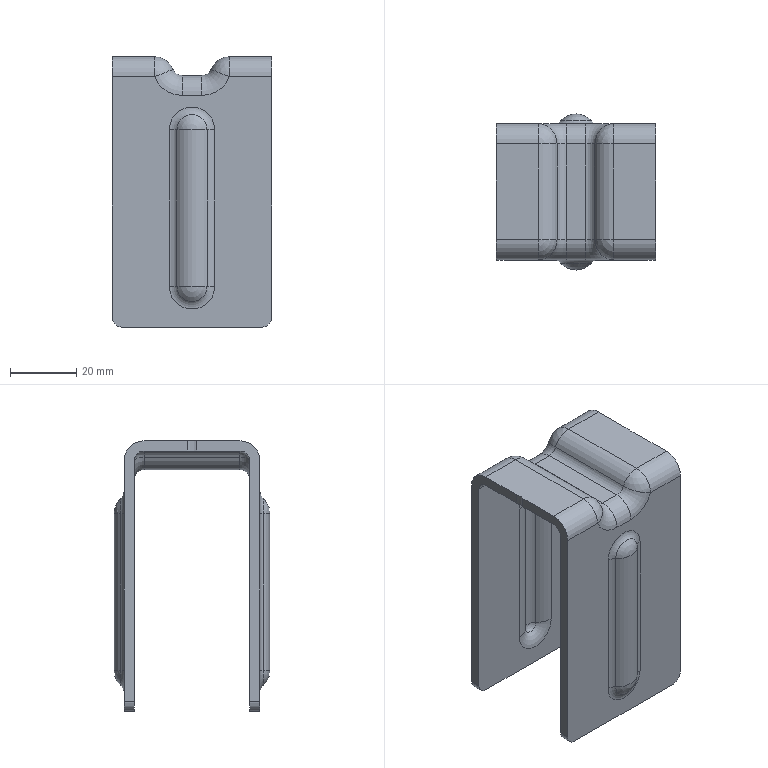Part | STEP file | PARTBODY_id330_x_t | 1 solid | 86 faces | box 48 x 46.9 x 81.415 mm | volume 29174 mm3 | cylinder 38 | plane 16 | torus 16 | sphere 16 | commonest cylinder face diameters 5.85 x10 12 x10 6.15 x6 12.3 x6 6 x4 9.576 x2